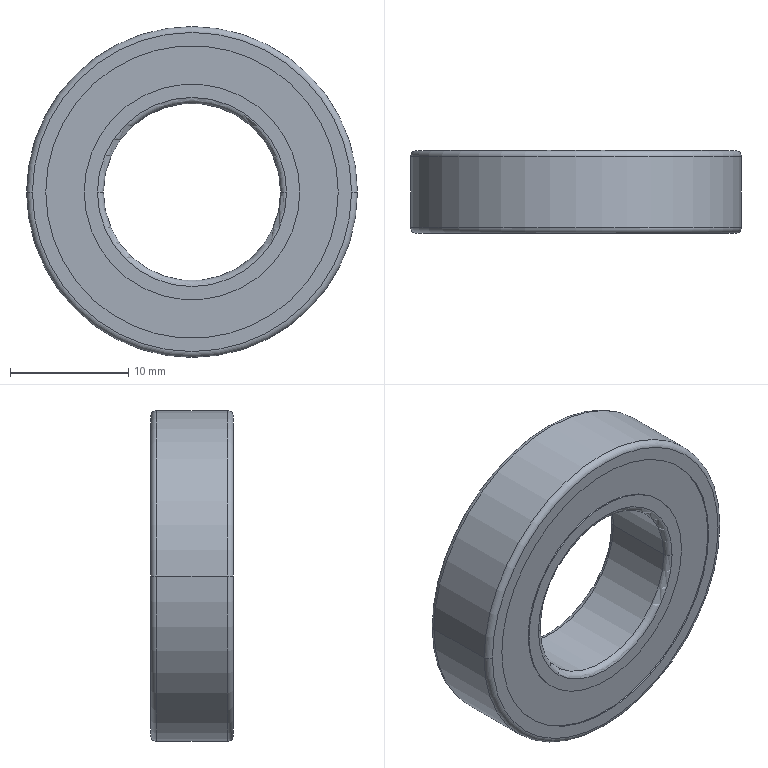Part | NX | 1 solid | 26 faces | box 28 x 7 x 28 mm | volume 3015 mm3 | cylinder 12 | torus 8 | plane 6 | commonest cylinder face diameters 18.25 x4 24.75 x4 15 x2 28 x2
STEP:
#1=CARTESIAN_POINT('',(7.5,3.,0.));
#2=VERTEX_POINT('',#1);
#3=CARTESIAN_POINT('',(-7.5,3.,0.));
#4=VERTEX_POINT('',#3);
#5=CARTESIAN_POINT('',(0.,3.,0.));
#6=DIRECTION('',(0.,-1.,0.));
#7=DIRECTION('',(-1.,0.,0.));
#8=AXIS2_PLACEMENT_3D('',#5,#6,#7);
#9=CIRCLE('',#8,7.5);
#10=EDGE_CURVE('',#2,#4,#9,.T.);
#11=ORIENTED_EDGE('',*,*,#10,.T.);
#12=CARTESIAN_POINT('',(-8.,3.5,0.));
#13=VERTEX_POINT('',#12);
#14=CARTESIAN_POINT('',(-8.,3.,0.));
#15=DIRECTION('',(0.,0.,-1.));
#16=DIRECTION('',(-1.,0.,0.));
#17=AXIS2_PLACEMENT_3D('',#14,#15,#16);
#18=CIRCLE('',#17,0.5);
#19=EDGE_CURVE('',#4,#13,#18,.F.);
#20=ORIENTED_EDGE('',*,*,#19,.T.);
#21=CARTESIAN_POINT('',(8.,3.5,0.));
#22=VERTEX_POINT('',#21);
#23=CARTESIAN_POINT('',(0.,3.5,0.));
#24=DIRECTION('',(0.,1.,0.));
#25=DIRECTION('',(1.,0.,0.));
#26=AXIS2_PLACEMENT_3D('',#23,#24,#25);
#27=CIRCLE('',#26,8.);
#28=EDGE_CURVE('',#13,#22,#27,.T.);
#29=ORIENTED_EDGE('',*,*,#28,.T.);
#30=CARTESIAN_POINT('',(8.,3.,0.));
#31=DIRECTION('',(0.,0.,1.));
#32=DIRECTION('',(1.,0.,0.));
#33=AXIS2_PLACEMENT_3D('',#30,#31,#32);
#34=CIRCLE('',#33,0.5);
#35=EDGE_CURVE('',#2,#22,#34,.F.);
#36=ORIENTED_EDGE('',*,*,#35,.F.);
#37=EDGE_LOOP('',(#11,#20,#29,#36));
#38=FACE_BOUND('',#37,.T.);
#39=CARTESIAN_POINT('',(0.,3.,0.));
#40=DIRECTION('',(0.,-1.,0.));
#41=DIRECTION('',(-1.,0.,0.));
#42=AXIS2_PLACEMENT_3D('',#39,#40,#41);
#43=TOROIDAL_SURFACE('',#42,8.,0.5);
#44=ADVANCED_FACE('',(#38),#43,.T.);
#45=CARTESIAN_POINT('',(14.,3.,0.));
#46=VERTEX_POINT('',#45);
#47=CARTESIAN_POINT('',(-14.,3.,0.));
#48=VERTEX_POINT('',#47);
#49=CARTESIAN_POINT('',(0.,3.,0.));
#50=DIRECTION('',(0.,-1.,0.));
#51=DIRECTION('',(-1.,0.,0.));
#52=AXIS2_PLACEMENT_3D('',#49,#50,#51);
#53=CIRCLE('',#52,14.);
#54=EDGE_CURVE('',#46,#48,#53,.T.);
#55=ORIENTED_EDGE('',*,*,#54,.F.);
#56=CARTESIAN_POINT('',(13.5,3.5,0.));
#57=VERTEX_POINT('',#56);
#58=CARTESIAN_POINT('',(13.5,3.,0.));
#59=DIRECTION('',(0.,0.,1.));
#60=DIRECTION('',(1.,0.,0.));
#61=AXIS2_PLACEMENT_3D('',#58,#59,#60);
#62=CIRCLE('',#61,0.5);
#63=EDGE_CURVE('',#57,#46,#62,.F.);
#64=ORIENTED_EDGE('',*,*,#63,.F.);
#65=CARTESIAN_POINT('',(-13.5,3.5,0.));
#66=VERTEX_POINT('',#65);
#67=CARTESIAN_POINT('',(0.,3.5,0.));
#68=DIRECTION('',(0.,-1.,0.));
#69=DIRECTION('',(1.,0.,0.));
#70=AXIS2_PLACEMENT_3D('',#67,#68,#69);
#71=CIRCLE('',#70,13.5);
#72=EDGE_CURVE('',#57,#66,#71,.T.);
#73=ORIENTED_EDGE('',*,*,#72,.T.);
#74=CARTESIAN_POINT('',(-13.5,3.,0.));
#75=DIRECTION('',(0.,0.,-1.));
#76=DIRECTION('',(-1.,0.,0.));
#77=AXIS2_PLACEMENT_3D('',#74,#75,#76);
#78=CIRCLE('',#77,0.5);
#79=EDGE_CURVE('',#66,#48,#78,.F.);
#80=ORIENTED_EDGE('',*,*,#79,.T.);
#81=EDGE_LOOP('',(#55,#64,#73,#80));
#82=FACE_BOUND('',#81,.T.);
#83=CARTESIAN_POINT('',(0.,3.,0.));
#84=DIRECTION('',(0.,-1.,0.));
#85=DIRECTION('',(-1.,0.,0.));
#86=AXIS2_PLACEMENT_3D('',#83,#84,#85);
#87=TOROIDAL_SURFACE('',#86,13.5,0.5);
#88=ADVANCED_FACE('',(#82),#87,.T.);
#89=CARTESIAN_POINT('',(-7.5,-3.,0.));
#90=VERTEX_POINT('',#89);
#91=CARTESIAN_POINT('',(7.5,-3.,0.));
#92=VERTEX_POINT('',#91);
#93=CARTESIAN_POINT('',(0.,-3.,0.));
#94=DIRECTION('',(0.,-1.,0.));
#95=DIRECTION('',(-1.,0.,0.));
#96=AXIS2_PLACEMENT_3D('',#93,#94,#95);
#97=CIRCLE('',#96,7.5);
#98=EDGE_CURVE('',#90,#92,#97,.T.);
#99=ORIENTED_EDGE('',*,*,#98,.T.);
#100=CARTESIAN_POINT('',(7.5,3.85,0.));
#101=DIRECTION('',(0.,-1.,0.));
#102=VECTOR('',#101,1000.);
#103=LINE('',#100,#102);
#104=EDGE_CURVE('',#2,#92,#103,.T.);
#105=ORIENTED_EDGE('',*,*,#104,.F.);
#106=CARTESIAN_POINT('',(0.,3.,0.));
#107=DIRECTION('',(0.,-1.,0.));
#108=DIRECTION('',(-1.,0.,0.));
#109=AXIS2_PLACEMENT_3D('',#106,#107,#108);
#110=CIRCLE('',#109,7.5);
#111=EDGE_CURVE('',#4,#2,#110,.T.);
#112=ORIENTED_EDGE('',*,*,#111,.F.);
#113=CARTESIAN_POINT('',(-7.5,3.85,0.));
#114=DIRECTION('',(0.,-1.,0.));
#115=VECTOR('',#114,1000.);
#116=LINE('',#113,#115);
#117=EDGE_CURVE('',#4,#90,#116,.T.);
#118=ORIENTED_EDGE('',*,*,#117,.T.);
#119=EDGE_LOOP('',(#99,#105,#112,#118));
#120=FACE_BOUND('',#119,.T.);
#121=CARTESIAN_POINT('',(0.,3.85,0.));
#122=DIRECTION('',(0.,-1.,0.));
#123=DIRECTION('',(-1.,0.,0.));
#124=AXIS2_PLACEMENT_3D('',#121,#122,#123);
#125=CYLINDRICAL_SURFACE('',#124,7.5);
#126=ADVANCED_FACE('',(#120),#125,.F.);
#127=CARTESIAN_POINT('',(-9.125,3.5,0.));
#128=VERTEX_POINT('',#127);
#129=CARTESIAN_POINT('',(9.125,3.5,0.));
#130=VERTEX_POINT('',#129);
#131=CARTESIAN_POINT('',(0.,3.5,0.));
#132=DIRECTION('',(0.,-1.,0.));
#133=DIRECTION('',(1.,0.,0.));
#134=AXIS2_PLACEMENT_3D('',#131,#132,#133);
#135=CIRCLE('',#134,9.125);
#136=EDGE_CURVE('',#128,#130,#135,.T.);
#137=ORIENTED_EDGE('',*,*,#136,.F.);
#138=CARTESIAN_POINT('',(0.,3.5,0.));
#139=DIRECTION('',(0.,-1.,0.));
#140=DIRECTION('',(1.,0.,0.));
#141=AXIS2_PLACEMENT_3D('',#138,#139,#140);
#142=CIRCLE('',#141,9.125);
#143=EDGE_CURVE('',#130,#128,#142,.T.);
#144=ORIENTED_EDGE('',*,*,#143,.F.);
#145=EDGE_LOOP('',(#137,#144));
#146=FACE_BOUND('',#145,.T.);
#147=ORIENTED_EDGE('',*,*,#28,.F.);
#148=CARTESIAN_POINT('',(0.,3.5,0.));
#149=DIRECTION('',(0.,1.,0.));
#150=DIRECTION('',(1.,0.,0.));
#151=AXIS2_PLACEMENT_3D('',#148,#149,#150);
#152=CIRCLE('',#151,8.);
#153=EDGE_CURVE('',#22,#13,#152,.T.);
#154=ORIENTED_EDGE('',*,*,#153,.F.);
#155=EDGE_LOOP('',(#147,#154));
#156=FACE_BOUND('',#155,.T.);
#157=CARTESIAN_POINT('',(0.,3.5,0.));
#158=DIRECTION('',(0.,-1.,0.));
#159=DIRECTION('',(0.,0.,-1.));
#160=AXIS2_PLACEMENT_3D('',#157,#158,#159);
#161=PLANE('',#160);
#162=ADVANCED_FACE('',(#146,#156),#161,.F.);
#163=CARTESIAN_POINT('',(8.,-3.5,0.));
#164=VERTEX_POINT('',#163);
#165=CARTESIAN_POINT('',(-8.,-3.5,0.));
#166=VERTEX_POINT('',#165);
#167=CARTESIAN_POINT('',(0.,-3.5,0.));
#168=DIRECTION('',(0.,-1.,0.));
#169=DIRECTION('',(1.,0.,0.));
#170=AXIS2_PLACEMENT_3D('',#167,#168,#169);
#171=CIRCLE('',#170,8.);
#172=EDGE_CURVE('',#164,#166,#171,.T.);
#173=ORIENTED_EDGE('',*,*,#172,.T.);
#174=CARTESIAN_POINT('',(-8.,-3.,0.));
#175=DIRECTION('',(0.,0.,-1.));
#176=DIRECTION('',(-1.,0.,0.));
#177=AXIS2_PLACEMENT_3D('',#174,#175,#176);
#178=CIRCLE('',#177,0.5);
#179=EDGE_CURVE('',#166,#90,#178,.F.);
#180=ORIENTED_EDGE('',*,*,#179,.T.);
#181=CARTESIAN_POINT('',(0.,-3.,0.));
#182=DIRECTION('',(0.,-1.,0.));
#183=DIRECTION('',(-1.,0.,0.));
#184=AXIS2_PLACEMENT_3D('',#181,#182,#183);
#185=CIRCLE('',#184,7.5);
#186=EDGE_CURVE('',#92,#90,#185,.T.);
#187=ORIENTED_EDGE('',*,*,#186,.F.);
#188=CARTESIAN_POINT('',(8.,-3.,0.));
#189=DIRECTION('',(0.,0.,1.));
#190=DIRECTION('',(1.,0.,0.));
#191=AXIS2_PLACEMENT_3D('',#188,#189,#190);
#192=CIRCLE('',#191,0.5);
#193=EDGE_CURVE('',#164,#92,#192,.F.);
#194=ORIENTED_EDGE('',*,*,#193,.F.);
#195=EDGE_LOOP('',(#173,#180,#187,#194));
#196=FACE_BOUND('',#195,.T.);
#197=CARTESIAN_POINT('',(0.,-3.,0.));
#198=DIRECTION('',(0.,-1.,0.));
#199=DIRECTION('',(-1.,0.,0.));
#200=AXIS2_PLACEMENT_3D('',#197,#198,#199);
#201=TOROIDAL_SURFACE('',#200,8.,0.5);
#202=ADVANCED_FACE('',(#196),#201,.T.);
#203=CARTESIAN_POINT('',(12.375,3.4,0.));
#204=VERTEX_POINT('',#203);
#205=CARTESIAN_POINT('',(-12.375,3.4,0.));
#206=VERTEX_POINT('',#205);
#207=CARTESIAN_POINT('',(0.,3.4,0.));
#208=DIRECTION('',(0.,-1.,0.));
#209=DIRECTION('',(1.,0.,0.));
#210=AXIS2_PLACEMENT_3D('',#207,#208,#209);
#211=CIRCLE('',#210,12.375);
#212=EDGE_CURVE('',#204,#206,#211,.T.);
#213=ORIENTED_EDGE('',*,*,#212,.F.);
#214=CARTESIAN_POINT('',(0.,3.4,0.));
#215=DIRECTION('',(0.,-1.,0.));
#216=DIRECTION('',(1.,0.,0.));
#217=AXIS2_PLACEMENT_3D('',#214,#215,#216);
#218=CIRCLE('',#217,12.375);
#219=EDGE_CURVE('',#206,#204,#218,.T.);
#220=ORIENTED_EDGE('',*,*,#219,.F.);
#221=EDGE_LOOP('',(#213,#220));
#222=FACE_BOUND('',#221,.T.);
#223=CARTESIAN_POINT('',(-9.125,3.4,0.));
#224=VERTEX_POINT('',#223);
#225=CARTESIAN_POINT('',(9.125,3.4,0.));
#226=VERTEX_POINT('',#225);
#227=CARTESIAN_POINT('',(0.,3.4,0.));
#228=DIRECTION('',(0.,1.,0.));
#229=DIRECTION('',(1.,0.,0.));
#230=AXIS2_PLACEMENT_3D('',#227,#228,#229);
#231=CIRCLE('',#230,9.125);
#232=EDGE_CURVE('',#224,#226,#231,.T.);
#233=ORIENTED_EDGE('',*,*,#232,.F.);
#234=CARTESIAN_POINT('',(0.,3.4,0.));
#235=DIRECTION('',(0.,1.,0.));
#236=DIRECTION('',(1.,0.,0.));
#237=AXIS2_PLACEMENT_3D('',#234,#235,#236);
#238=CIRCLE('',#237,9.125);
#239=EDGE_CURVE('',#226,#224,#238,.T.);
#240=ORIENTED_EDGE('',*,*,#239,.F.);
#241=EDGE_LOOP('',(#233,#240));
#242=FACE_BOUND('',#241,.T.);
#243=CARTESIAN_POINT('',(0.,3.4,0.));
#244=DIRECTION('',(0.,-1.,0.));
#245=DIRECTION('',(0.,0.,-1.));
#246=AXIS2_PLACEMENT_3D('',#243,#244,#245);
#247=PLANE('',#246);
#248=ADVANCED_FACE('',(#222,#242),#247,.F.);
#249=CARTESIAN_POINT('',(9.125,-3.5,0.));
#250=VERTEX_POINT('',#249);
#251=CARTESIAN_POINT('',(-9.125,-3.5,0.));
#252=VERTEX_POINT('',#251);
#253=CARTESIAN_POINT('',(0.,-3.5,0.));
#254=DIRECTION('',(0.,1.,0.));
#255=DIRECTION('',(1.,0.,0.));
#256=AXIS2_PLACEMENT_3D('',#253,#254,#255);
#257=CIRCLE('',#256,9.125);
#258=EDGE_CURVE('',#250,#252,#257,.T.);
#259=ORIENTED_EDGE('',*,*,#258,.F.);
#260=CARTESIAN_POINT('',(0.,-3.5,0.));
#261=DIRECTION('',(0.,1.,0.));
#262=DIRECTION('',(1.,0.,0.));
#263=AXIS2_PLACEMENT_3D('',#260,#261,#262);
#264=CIRCLE('',#263,9.125);
#265=EDGE_CURVE('',#252,#250,#264,.T.);
#266=ORIENTED_EDGE('',*,*,#265,.F.);
#267=EDGE_LOOP('',(#259,#266));
#268=FACE_BOUND('',#267,.T.);
#269=ORIENTED_EDGE('',*,*,#172,.F.);
#270=CARTESIAN_POINT('',(0.,-3.5,0.));
#271=DIRECTION('',(0.,-1.,0.));
#272=DIRECTION('',(1.,0.,0.));
#273=AXIS2_PLACEMENT_3D('',#270,#271,#272);
#274=CIRCLE('',#273,8.);
#275=EDGE_CURVE('',#166,#164,#274,.T.);
#276=ORIENTED_EDGE('',*,*,#275,.F.);
#277=EDGE_LOOP('',(#269,#276));
#278=FACE_BOUND('',#277,.T.);
#279=CARTESIAN_POINT('',(0.,-3.5,0.));
#280=DIRECTION('',(0.,-1.,0.));
#281=DIRECTION('',(0.,0.,-1.));
#282=AXIS2_PLACEMENT_3D('',#279,#280,#281);
#283=PLANE('',#282);
#284=ADVANCED_FACE('',(#268,#278),#283,.T.);
#285=ORIENTED_EDGE('',*,*,#258,.T.);
#286=CARTESIAN_POINT('',(-9.125,-3.4,0.));
#287=VERTEX_POINT('',#286);
#288=CARTESIAN_POINT('',(-9.125,3.85,0.));
#289=DIRECTION('',(0.,-1.,0.));
#290=VECTOR('',#289,1000.);
#291=LINE('',#288,#290);
#292=EDGE_CURVE('',#252,#287,#291,.F.);
#293=ORIENTED_EDGE('',*,*,#292,.T.);
#294=CARTESIAN_POINT('',(9.125,-3.4,0.));
#295=VERTEX_POINT('',#294);
#296=CARTESIAN_POINT('',(0.,-3.4,0.));
#297=DIRECTION('',(0.,-1.,0.));
#298=DIRECTION('',(1.,0.,0.));
#299=AXIS2_PLACEMENT_3D('',#296,#297,#298);
#300=CIRCLE('',#299,9.125);
#301=EDGE_CURVE('',#287,#295,#300,.T.);
#302=ORIENTED_EDGE('',*,*,#301,.T.);
#303=CARTESIAN_POINT('',(9.125,3.85,0.));
#304=DIRECTION('',(0.,-1.,0.));
#305=VECTOR('',#304,1000.);
#306=LINE('',#303,#305);
#307=EDGE_CURVE('',#250,#295,#306,.F.);
#308=ORIENTED_EDGE('',*,*,#307,.F.);
#309=EDGE_LOOP('',(#285,#293,#302,#308));
#310=FACE_BOUND('',#309,.T.);
#311=CARTESIAN_POINT('',(0.,3.85,0.));
#312=DIRECTION('',(0.,-1.,0.));
#313=DIRECTION('',(-1.,0.,0.));
#314=AXIS2_PLACEMENT_3D('',#311,#312,#313);
#315=CYLINDRICAL_SURFACE('',#314,9.125);
#316=ADVANCED_FACE('',(#310),#315,.T.);
#317=CARTESIAN_POINT('',(-12.375,3.5,0.));
#318=VERTEX_POINT('',#317);
#319=CARTESIAN_POINT('',(12.375,3.5,0.));
#320=VERTEX_POINT('',#319);
#321=CARTESIAN_POINT('',(0.,3.5,0.));
#322=DIRECTION('',(0.,1.,0.));
#323=DIRECTION('',(1.,0.,0.));
#324=AXIS2_PLACEMENT_3D('',#321,#322,#323);
#325=CIRCLE('',#324,12.375);
#326=EDGE_CURVE('',#318,#320,#325,.T.);
#327=ORIENTED_EDGE('',*,*,#326,.T.);
#328=CARTESIAN_POINT('',(12.375,3.85,0.));
#329=DIRECTION('',(0.,-1.,0.));
#330=VECTOR('',#329,1000.);
#331=LINE('',#328,#330);
#332=EDGE_CURVE('',#204,#320,#331,.F.);
#333=ORIENTED_EDGE('',*,*,#332,.F.);
#334=ORIENTED_EDGE('',*,*,#212,.T.);
#335=CARTESIAN_POINT('',(-12.375,3.85,0.));
#336=DIRECTION('',(0.,-1.,0.));
#337=VECTOR('',#336,1000.);
#338=LINE('',#335,#337);
#339=EDGE_CURVE('',#206,#318,#338,.F.);
#340=ORIENTED_EDGE('',*,*,#339,.T.);
#341=EDGE_LOOP('',(#327,#333,#334,#340));
#342=FACE_BOUND('',#341,.T.);
#343=CARTESIAN_POINT('',(0.,3.85,0.));
#344=DIRECTION('',(0.,-1.,0.));
#345=DIRECTION('',(-1.,0.,0.));
#346=AXIS2_PLACEMENT_3D('',#343,#344,#345);
#347=CYLINDRICAL_SURFACE('',#346,12.375);
#348=ADVANCED_FACE('',(#342),#347,.F.);
#349=CARTESIAN_POINT('',(-12.375,-3.4,0.));
#350=VERTEX_POINT('',#349);
#351=CARTESIAN_POINT('',(12.375,-3.4,0.));
#352=VERTEX_POINT('',#351);
#353=CARTESIAN_POINT('',(0.,-3.4,0.));
#354=DIRECTION('',(0.,1.,0.));
#355=DIRECTION('',(1.,0.,0.));
#356=AXIS2_PLACEMENT_3D('',#353,#354,#355);
#357=CIRCLE('',#356,12.375);
#358=EDGE_CURVE('',#350,#352,#357,.T.);
#359=ORIENTED_EDGE('',*,*,#358,.F.);
#360=CARTESIAN_POINT('',(0.,-3.4,0.));
#361=DIRECTION('',(0.,1.,0.));
#362=DIRECTION('',(1.,0.,0.));
#363=AXIS2_PLACEMENT_3D('',#360,#361,#362);
#364=CIRCLE('',#363,12.375);
#365=EDGE_CURVE('',#352,#350,#364,.T.);
#366=ORIENTED_EDGE('',*,*,#365,.F.);
#367=EDGE_LOOP('',(#359,#366));
#368=FACE_BOUND('',#367,.T.);
#369=CARTESIAN_POINT('',(0.,-3.4,0.));
#370=DIRECTION('',(0.,-1.,0.));
#371=DIRECTION('',(1.,0.,0.));
#372=AXIS2_PLACEMENT_3D('',#369,#370,#371);
#373=CIRCLE('',#372,9.125);
#374=EDGE_CURVE('',#295,#287,#373,.T.);
#375=ORIENTED_EDGE('',*,*,#374,.F.);
#376=ORIENTED_EDGE('',*,*,#301,.F.);
#377=EDGE_LOOP('',(#375,#376));
#378=FACE_BOUND('',#377,.T.);
#379=CARTESIAN_POINT('',(0.,-3.4,0.));
#380=DIRECTION('',(0.,-1.,0.));
#381=DIRECTION('',(0.,0.,-1.));
#382=AXIS2_PLACEMENT_3D('',#379,#380,#381);
#383=PLANE('',#382);
#384=ADVANCED_FACE('',(#368,#378),#383,.T.);
#385=ORIENTED_EDGE('',*,*,#358,.T.);
#386=CARTESIAN_POINT('',(12.375,-3.5,0.));
#387=VERTEX_POINT('',#386);
#388=CARTESIAN_POINT('',(12.375,3.85,0.));
#389=DIRECTION('',(0.,-1.,0.));
#390=VECTOR('',#389,1000.);
#391=LINE('',#388,#390);
#392=EDGE_CURVE('',#387,#352,#391,.F.);
#393=ORIENTED_EDGE('',*,*,#392,.F.);
#394=CARTESIAN_POINT('',(-12.375,-3.5,0.));
#395=VERTEX_POINT('',#394);
#396=CARTESIAN_POINT('',(0.,-3.5,0.));
#397=DIRECTION('',(0.,-1.,0.));
#398=DIRECTION('',(1.,0.,0.));
#399=AXIS2_PLACEMENT_3D('',#396,#397,#398);
#400=CIRCLE('',#399,12.375);
#401=EDGE_CURVE('',#387,#395,#400,.T.);
#402=ORIENTED_EDGE('',*,*,#401,.T.);
#403=CARTESIAN_POINT('',(-12.375,3.85,0.));
#404=DIRECTION('',(0.,-1.,0.));
#405=VECTOR('',#404,1000.);
#406=LINE('',#403,#405);
#407=EDGE_CURVE('',#395,#350,#406,.F.);
#408=ORIENTED_EDGE('',*,*,#407,.T.);
#409=EDGE_LOOP('',(#385,#393,#402,#408));
#410=FACE_BOUND('',#409,.T.);
#411=CARTESIAN_POINT('',(0.,3.85,0.));
#412=DIRECTION('',(0.,-1.,0.));
#413=DIRECTION('',(-1.,0.,0.));
#414=AXIS2_PLACEMENT_3D('',#411,#412,#413);
#415=CYLINDRICAL_SURFACE('',#414,12.375);
#416=ADVANCED_FACE('',(#410),#415,.F.);
#417=ORIENTED_EDGE('',*,*,#232,.T.);
#418=CARTESIAN_POINT('',(9.125,3.85,0.));
#419=DIRECTION('',(0.,-1.,0.));
#420=VECTOR('',#419,1000.);
#421=LINE('',#418,#420);
#422=EDGE_CURVE('',#130,#226,#421,.T.);
#423=ORIENTED_EDGE('',*,*,#422,.F.);
#424=ORIENTED_EDGE('',*,*,#143,.T.);
#425=CARTESIAN_POINT('',(-9.125,3.85,0.));
#426=DIRECTION('',(0.,-1.,0.));
#427=VECTOR('',#426,1000.);
#428=LINE('',#425,#427);
#429=EDGE_CURVE('',#128,#224,#428,.T.);
#430=ORIENTED_EDGE('',*,*,#429,.T.);
#431=EDGE_LOOP('',(#417,#423,#424,#430));
#432=FACE_BOUND('',#431,.T.);
#433=CARTESIAN_POINT('',(0.,3.85,0.));
#434=DIRECTION('',(0.,-1.,0.));
#435=DIRECTION('',(-1.,0.,0.));
#436=AXIS2_PLACEMENT_3D('',#433,#434,#435);
#437=CYLINDRICAL_SURFACE('',#436,9.125);
#438=ADVANCED_FACE('',(#432),#437,.T.);
#439=CARTESIAN_POINT('',(-13.5,-3.5,0.));
#440=VERTEX_POINT('',#439);
#441=CARTESIAN_POINT('',(13.5,-3.5,0.));
#442=VERTEX_POINT('',#441);
#443=CARTESIAN_POINT('',(0.,-3.5,0.));
#444=DIRECTION('',(0.,1.,0.));
#445=DIRECTION('',(1.,0.,0.));
#446=AXIS2_PLACEMENT_3D('',#443,#444,#445);
#447=CIRCLE('',#446,13.5);
#448=EDGE_CURVE('',#440,#442,#447,.T.);
#449=ORIENTED_EDGE('',*,*,#448,.F.);
#450=CARTESIAN_POINT('',(0.,-3.5,0.));
#451=DIRECTION('',(0.,1.,0.));
#452=DIRECTION('',(1.,0.,0.));
#453=AXIS2_PLACEMENT_3D('',#450,#451,#452);
#454=CIRCLE('',#453,13.5);
#455=EDGE_CURVE('',#442,#440,#454,.T.);
#456=ORIENTED_EDGE('',*,*,#455,.F.);
#457=EDGE_LOOP('',(#449,#456));
#458=FACE_BOUND('',#457,.T.);
#459=ORIENTED_EDGE('',*,*,#401,.F.);
#460=CARTESIAN_POINT('',(0.,-3.5,0.));
#461=DIRECTION('',(0.,-1.,0.));
#462=DIRECTION('',(1.,0.,0.));
#463=AXIS2_PLACEMENT_3D('',#460,#461,#462);
#464=CIRCLE('',#463,12.375);
#465=EDGE_CURVE('',#395,#387,#464,.T.);
#466=ORIENTED_EDGE('',*,*,#465,.F.);
#467=EDGE_LOOP('',(#459,#466));
#468=FACE_BOUND('',#467,.T.);
#469=CARTESIAN_POINT('',(0.,-3.5,0.));
#470=DIRECTION('',(0.,-1.,0.));
#471=DIRECTION('',(0.,0.,-1.));
#472=AXIS2_PLACEMENT_3D('',#469,#470,#471);
#473=PLANE('',#472);
#474=ADVANCED_FACE('',(#458,#468),#473,.T.);
#475=ORIENTED_EDGE('',*,*,#448,.T.);
#476=CARTESIAN_POINT('',(14.,-3.,0.));
#477=VERTEX_POINT('',#476);
#478=CARTESIAN_POINT('',(13.5,-3.,0.));
#479=DIRECTION('',(0.,0.,1.));
#480=DIRECTION('',(1.,0.,0.));
#481=AXIS2_PLACEMENT_3D('',#478,#479,#480);
#482=CIRCLE('',#481,0.5);
#483=EDGE_CURVE('',#477,#442,#482,.F.);
#484=ORIENTED_EDGE('',*,*,#483,.F.);
#485=CARTESIAN_POINT('',(-14.,-3.,0.));
#486=VERTEX_POINT('',#485);
#487=CARTESIAN_POINT('',(0.,-3.,0.));
#488=DIRECTION('',(0.,-1.,0.));
#489=DIRECTION('',(-1.,0.,0.));
#490=AXIS2_PLACEMENT_3D('',#487,#488,#489);
#491=CIRCLE('',#490,14.);
#492=EDGE_CURVE('',#477,#486,#491,.T.);
#493=ORIENTED_EDGE('',*,*,#492,.T.);
#494=CARTESIAN_POINT('',(-13.5,-3.,0.));
#495=DIRECTION('',(0.,0.,-1.));
#496=DIRECTION('',(-1.,0.,0.));
#497=AXIS2_PLACEMENT_3D('',#494,#495,#496);
#498=CIRCLE('',#497,0.5);
#499=EDGE_CURVE('',#486,#440,#498,.F.);
#500=ORIENTED_EDGE('',*,*,#499,.T.);
#501=EDGE_LOOP('',(#475,#484,#493,#500));
#502=FACE_BOUND('',#501,.T.);
#503=CARTESIAN_POINT('',(0.,-3.,0.));
#504=DIRECTION('',(0.,-1.,0.));
#505=DIRECTION('',(-1.,0.,0.));
#506=AXIS2_PLACEMENT_3D('',#503,#504,#505);
#507=TOROIDAL_SURFACE('',#506,13.5,0.5);
#508=ADVANCED_FACE('',(#502),#507,.T.);
#509=ORIENTED_EDGE('',*,*,#72,.F.);
#510=CARTESIAN_POINT('',(0.,3.5,0.));
#511=DIRECTION('',(0.,-1.,0.));
#512=DIRECTION('',(1.,0.,0.));
#513=AXIS2_PLACEMENT_3D('',#510,#511,#512);
#514=CIRCLE('',#513,13.5);
#515=EDGE_CURVE('',#66,#57,#514,.T.);
#516=ORIENTED_EDGE('',*,*,#515,.F.);
#517=EDGE_LOOP('',(#509,#516));
#518=FACE_BOUND('',#517,.T.);
#519=ORIENTED_EDGE('',*,*,#326,.F.);
#520=CARTESIAN_POINT('',(0.,3.5,0.));
#521=DIRECTION('',(0.,1.,0.));
#522=DIRECTION('',(1.,0.,0.));
#523=AXIS2_PLACEMENT_3D('',#520,#521,#522);
#524=CIRCLE('',#523,12.375);
#525=EDGE_CURVE('',#320,#318,#524,.T.);
#526=ORIENTED_EDGE('',*,*,#525,.F.);
#527=EDGE_LOOP('',(#519,#526));
#528=FACE_BOUND('',#527,.T.);
#529=CARTESIAN_POINT('',(0.,3.5,0.));
#530=DIRECTION('',(0.,-1.,0.));
#531=DIRECTION('',(0.,0.,-1.));
#532=AXIS2_PLACEMENT_3D('',#529,#530,#531);
#533=PLANE('',#532);
#534=ADVANCED_FACE('',(#518,#528),#533,.F.);
#535=ORIENTED_EDGE('',*,*,#492,.F.);
#536=CARTESIAN_POINT('',(14.,3.85,0.));
#537=DIRECTION('',(0.,-1.,0.));
#538=VECTOR('',#537,1000.);
#539=LINE('',#536,#538);
#540=EDGE_CURVE('',#477,#46,#539,.F.);
#541=ORIENTED_EDGE('',*,*,#540,.T.);
#542=ORIENTED_EDGE('',*,*,#54,.T.);
#543=CARTESIAN_POINT('',(-14.,3.85,0.));
#544=DIRECTION('',(0.,-1.,0.));
#545=VECTOR('',#544,1000.);
#546=LINE('',#543,#545);
#547=EDGE_CURVE('',#486,#48,#546,.F.);
#548=ORIENTED_EDGE('',*,*,#547,.F.);
#549=EDGE_LOOP('',(#535,#541,#542,#548));
#550=FACE_BOUND('',#549,.T.);
#551=CARTESIAN_POINT('',(0.,3.85,0.));
#552=DIRECTION('',(0.,-1.,0.));
#553=DIRECTION('',(-1.,0.,0.));
#554=AXIS2_PLACEMENT_3D('',#551,#552,#553);
#555=CYLINDRICAL_SURFACE('',#554,14.);
#556=ADVANCED_FACE('',(#550),#555,.T.);
#557=ORIENTED_EDGE('',*,*,#339,.F.);
#558=ORIENTED_EDGE('',*,*,#219,.T.);
#559=ORIENTED_EDGE('',*,*,#332,.T.);
#560=ORIENTED_EDGE('',*,*,#525,.T.);
#561=EDGE_LOOP('',(#557,#558,#559,#560));
#562=FACE_BOUND('',#561,.T.);
#563=CARTESIAN_POINT('',(0.,3.85,0.));
#564=DIRECTION('',(0.,-1.,0.));
#565=DIRECTION('',(-1.,0.,0.));
#566=AXIS2_PLACEMENT_3D('',#563,#564,#565);
#567=CYLINDRICAL_SURFACE('',#566,12.375);
#568=ADVANCED_FACE('',(#562),#567,.F.);
#569=ORIENTED_EDGE('',*,*,#374,.T.);
#570=ORIENTED_EDGE('',*,*,#292,.F.);
#571=ORIENTED_EDGE('',*,*,#265,.T.);
#572=ORIENTED_EDGE('',*,*,#307,.T.);
#573=EDGE_LOOP('',(#569,#570,#571,#572));
#574=FACE_BOUND('',#573,.T.);
#575=CARTESIAN_POINT('',(0.,3.85,0.));
#576=DIRECTION('',(0.,-1.,0.));
#577=DIRECTION('',(-1.,0.,0.));
#578=AXIS2_PLACEMENT_3D('',#575,#576,#577);
#579=CYLINDRICAL_SURFACE('',#578,9.125);
#580=ADVANCED_FACE('',(#574),#579,.T.);
#581=ORIENTED_EDGE('',*,*,#547,.T.);
#582=CARTESIAN_POINT('',(0.,3.,0.));
#583=DIRECTION('',(0.,-1.,0.));
#584=DIRECTION('',(-1.,0.,0.));
#585=AXIS2_PLACEMENT_3D('',#582,#583,#584);
#586=CIRCLE('',#585,14.);
#587=EDGE_CURVE('',#48,#46,#586,.T.);
#588=ORIENTED_EDGE('',*,*,#587,.T.);
#589=ORIENTED_EDGE('',*,*,#540,.F.);
#590=CARTESIAN_POINT('',(0.,-3.,0.));
#591=DIRECTION('',(0.,-1.,0.));
#592=DIRECTION('',(-1.,0.,0.));
#593=AXIS2_PLACEMENT_3D('',#590,#591,#592);
#594=CIRCLE('',#593,14.);
#595=EDGE_CURVE('',#486,#477,#594,.T.);
#596=ORIENTED_EDGE('',*,*,#595,.F.);
#597=EDGE_LOOP('',(#581,#588,#589,#596));
#598=FACE_BOUND('',#597,.T.);
#599=CARTESIAN_POINT('',(0.,3.85,0.));
#600=DIRECTION('',(0.,-1.,0.));
#601=DIRECTION('',(-1.,0.,0.));
#602=AXIS2_PLACEMENT_3D('',#599,#600,#601);
#603=CYLINDRICAL_SURFACE('',#602,14.);
#604=ADVANCED_FACE('',(#598),#603,.T.);
#605=ORIENTED_EDGE('',*,*,#10,.F.);
#606=ORIENTED_EDGE('',*,*,#104,.T.);
#607=ORIENTED_EDGE('',*,*,#186,.T.);
#608=ORIENTED_EDGE('',*,*,#117,.F.);
#609=EDGE_LOOP('',(#605,#606,#607,#608));
#610=FACE_BOUND('',#609,.T.);
#611=CARTESIAN_POINT('',(0.,3.85,0.));
#612=DIRECTION('',(0.,-1.,0.));
#613=DIRECTION('',(-1.,0.,0.));
#614=AXIS2_PLACEMENT_3D('',#611,#612,#613);
#615=CYLINDRICAL_SURFACE('',#614,7.5);
#616=ADVANCED_FACE('',(#610),#615,.F.);
#617=ORIENTED_EDGE('',*,*,#136,.T.);
#618=ORIENTED_EDGE('',*,*,#422,.T.);
#619=ORIENTED_EDGE('',*,*,#239,.T.);
#620=ORIENTED_EDGE('',*,*,#429,.F.);
#621=EDGE_LOOP('',(#617,#618,#619,#620));
#622=FACE_BOUND('',#621,.T.);
#623=CARTESIAN_POINT('',(0.,3.85,0.));
#624=DIRECTION('',(0.,-1.,0.));
#625=DIRECTION('',(-1.,0.,0.));
#626=AXIS2_PLACEMENT_3D('',#623,#624,#625);
#627=CYLINDRICAL_SURFACE('',#626,9.125);
#628=ADVANCED_FACE('',(#622),#627,.T.);
#629=ORIENTED_EDGE('',*,*,#407,.F.);
#630=ORIENTED_EDGE('',*,*,#465,.T.);
#631=ORIENTED_EDGE('',*,*,#392,.T.);
#632=ORIENTED_EDGE('',*,*,#365,.T.);
#633=EDGE_LOOP('',(#629,#630,#631,#632));
#634=FACE_BOUND('',#633,.T.);
#635=CARTESIAN_POINT('',(0.,3.85,0.));
#636=DIRECTION('',(0.,-1.,0.));
#637=DIRECTION('',(-1.,0.,0.));
#638=AXIS2_PLACEMENT_3D('',#635,#636,#637);
#639=CYLINDRICAL_SURFACE('',#638,12.375);
#640=ADVANCED_FACE('',(#634),#639,.F.);
#641=ORIENTED_EDGE('',*,*,#79,.F.);
#642=ORIENTED_EDGE('',*,*,#515,.T.);
#643=ORIENTED_EDGE('',*,*,#63,.T.);
#644=ORIENTED_EDGE('',*,*,#587,.F.);
#645=EDGE_LOOP('',(#641,#642,#643,#644));
#646=FACE_BOUND('',#645,.T.);
#647=CARTESIAN_POINT('',(0.,3.,0.));
#648=DIRECTION('',(0.,-1.,0.));
#649=DIRECTION('',(-1.,0.,0.));
#650=AXIS2_PLACEMENT_3D('',#647,#648,#649);
#651=TOROIDAL_SURFACE('',#650,13.5,0.5);
#652=ADVANCED_FACE('',(#646),#651,.T.);
#653=ORIENTED_EDGE('',*,*,#98,.F.);
#654=ORIENTED_EDGE('',*,*,#179,.F.);
#655=ORIENTED_EDGE('',*,*,#275,.T.);
#656=ORIENTED_EDGE('',*,*,#193,.T.);
#657=EDGE_LOOP('',(#653,#654,#655,#656));
#658=FACE_BOUND('',#657,.T.);
#659=CARTESIAN_POINT('',(0.,-3.,0.));
#660=DIRECTION('',(0.,-1.,0.));
#661=DIRECTION('',(-1.,0.,0.));
#662=AXIS2_PLACEMENT_3D('',#659,#660,#661);
#663=TOROIDAL_SURFACE('',#662,8.,0.5);
#664=ADVANCED_FACE('',(#658),#663,.T.);
#665=ORIENTED_EDGE('',*,*,#499,.F.);
#666=ORIENTED_EDGE('',*,*,#595,.T.);
#667=ORIENTED_EDGE('',*,*,#483,.T.);
#668=ORIENTED_EDGE('',*,*,#455,.T.);
#669=EDGE_LOOP('',(#665,#666,#667,#668));
#670=FACE_BOUND('',#669,.T.);
#671=CARTESIAN_POINT('',(0.,-3.,0.));
#672=DIRECTION('',(0.,-1.,0.));
#673=DIRECTION('',(-1.,0.,0.));
#674=AXIS2_PLACEMENT_3D('',#671,#672,#673);
#675=TOROIDAL_SURFACE('',#674,13.5,0.5);
#676=ADVANCED_FACE('',(#670),#675,.T.);
#677=ORIENTED_EDGE('',*,*,#19,.F.);
#678=ORIENTED_EDGE('',*,*,#111,.T.);
#679=ORIENTED_EDGE('',*,*,#35,.T.);
#680=ORIENTED_EDGE('',*,*,#153,.T.);
#681=EDGE_LOOP('',(#677,#678,#679,#680));
#682=FACE_BOUND('',#681,.T.);
#683=CARTESIAN_POINT('',(0.,3.,0.));
#684=DIRECTION('',(0.,-1.,0.));
#685=DIRECTION('',(-1.,0.,0.));
#686=AXIS2_PLACEMENT_3D('',#683,#684,#685);
#687=TOROIDAL_SURFACE('',#686,8.,0.5);
#688=ADVANCED_FACE('',(#682),#687,.T.);
#689=CLOSED_SHELL('',(#44,#88,#126,#162,#202,#248,#284,#316,#348,#384,#416,#438,#474,#508,#534,#556,#568,#580,#604,#616,#628,#640,#652,#664,#676,#688));
#690=MANIFOLD_SOLID_BREP('',#689);
#691=(LENGTH_UNIT()NAMED_UNIT(*)SI_UNIT(.MILLI.,.METRE.));
#692=UNCERTAINTY_MEASURE_WITH_UNIT(LENGTH_MEASURE(0.00001),#691,'','');
#693=(NAMED_UNIT(*)PLANE_ANGLE_UNIT()SI_UNIT($,.RADIAN.));
#694=(NAMED_UNIT(*)SI_UNIT($,.STERADIAN.)SOLID_ANGLE_UNIT());
#695=(GEOMETRIC_REPRESENTATION_CONTEXT(3)GLOBAL_UNCERTAINTY_ASSIGNED_CONTEXT((#692))GLOBAL_UNIT_ASSIGNED_CONTEXT((#691,#693,#694))REPRESENTATION_CONTEXT('',''));
#696=ADVANCED_BREP_SHAPE_REPRESENTATION('',(#690),#695);